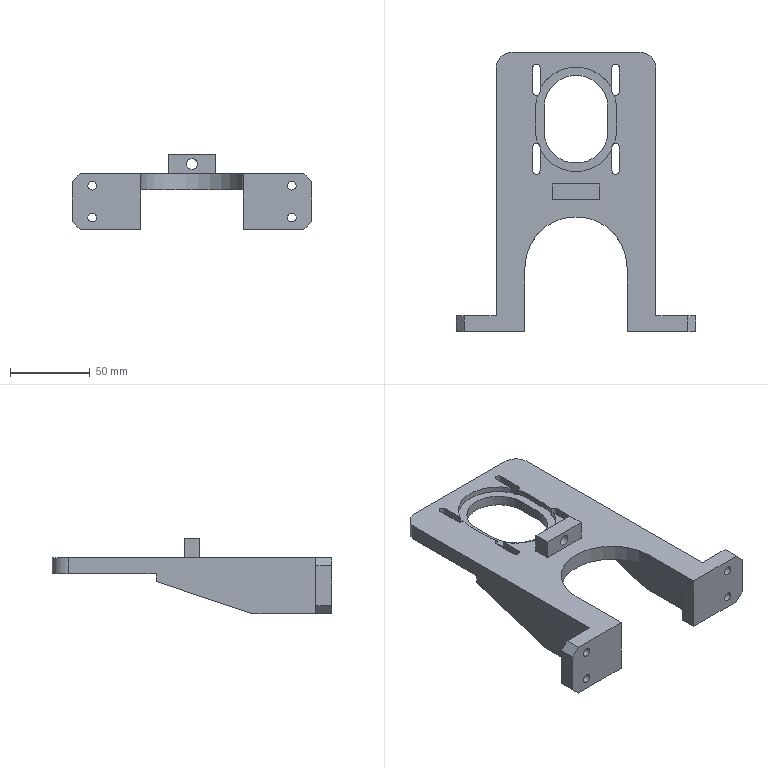Part | NX | 1 solid | 97 faces | box 150 x 175 x 47 mm | volume 171478 mm3 | plane 61 | cylinder 36 | commonest cylinder face diameters 4.5 x8 8.2 x8 50.5 x6 5.5 x4 10 x4 20 x2